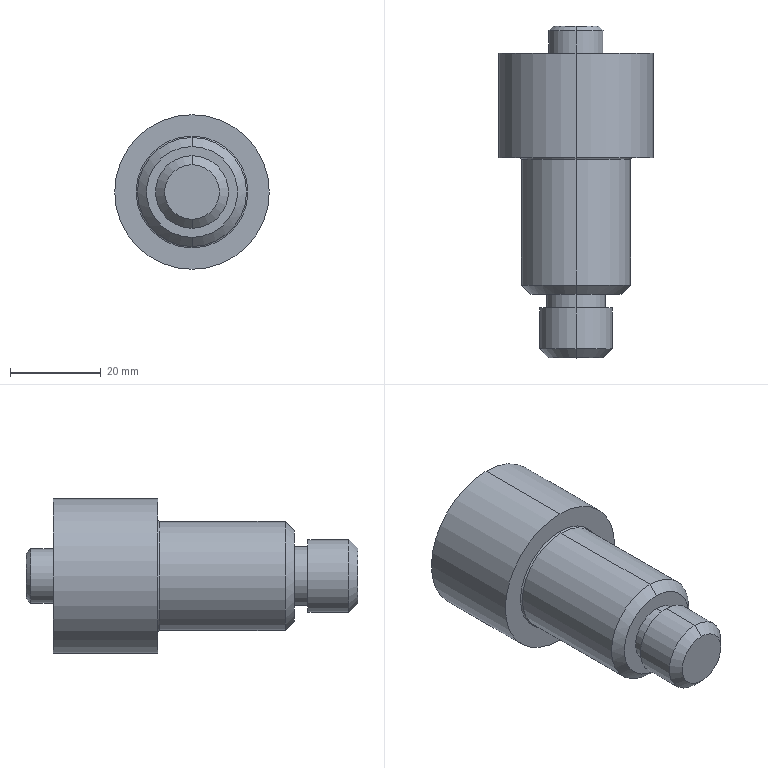Part | SolidWorks | features MirrorStock 1 | 1 solid | 24 faces | box 34 x 73 x 34 mm | volume 37491 mm3 | cylinder 10 | cone 6 | plane 6 | torus 2 | commonest cylinder face diameters 12 x2 13 x2 16 x2 24 x2 34 x2
STEP:
#1=CARTESIAN_POINT('',(0.,-29.3,12.));
#2=VERTEX_POINT('',#1);
#3=CARTESIAN_POINT('',(0.,-29.3,-12.));
#4=VERTEX_POINT('',#3);
#5=CARTESIAN_POINT('',(0.,-29.3,0.));
#6=DIRECTION('',(0.,1.,0.));
#7=DIRECTION('',(0.,0.,1.));
#8=AXIS2_PLACEMENT_3D('',#5,#6,#7);
#9=CIRCLE('',#8,12.);
#10=EDGE_CURVE('',#2,#4,#9,.T.);
#11=ORIENTED_EDGE('',*,*,#10,.T.);
#12=CARTESIAN_POINT('',(0.,-29.,-12.3));
#13=VERTEX_POINT('',#12);
#14=CARTESIAN_POINT('',(0.,-29.3,-12.3));
#15=DIRECTION('',(-1.,0.,0.));
#16=DIRECTION('',(0.,0.,1.));
#17=AXIS2_PLACEMENT_3D('',#14,#15,#16);
#18=CIRCLE('',#17,0.3);
#19=EDGE_CURVE('',#4,#13,#18,.T.);
#20=ORIENTED_EDGE('',*,*,#19,.T.);
#21=CARTESIAN_POINT('',(0.,-29.,12.3));
#22=VERTEX_POINT('',#21);
#23=CARTESIAN_POINT('',(0.,-29.,0.));
#24=DIRECTION('',(0.,-1.,0.));
#25=DIRECTION('',(0.,0.,1.));
#26=AXIS2_PLACEMENT_3D('',#23,#24,#25);
#27=CIRCLE('',#26,12.3);
#28=EDGE_CURVE('',#13,#22,#27,.T.);
#29=ORIENTED_EDGE('',*,*,#28,.T.);
#30=CARTESIAN_POINT('',(0.,-29.3,12.3));
#31=DIRECTION('',(1.,0.,0.));
#32=DIRECTION('',(0.,0.,-1.));
#33=AXIS2_PLACEMENT_3D('',#30,#31,#32);
#34=CIRCLE('',#33,0.3);
#35=EDGE_CURVE('',#2,#22,#34,.T.);
#36=ORIENTED_EDGE('',*,*,#35,.F.);
#37=EDGE_LOOP('',(#11,#20,#29,#36));
#38=FACE_OUTER_BOUND('',#37,.T.);
#39=CARTESIAN_POINT('',(0.,-29.3,0.));
#40=DIRECTION('',(0.,-1.,0.));
#41=DIRECTION('',(0.,0.,1.));
#42=AXIS2_PLACEMENT_3D('',#39,#40,#41);
#43=TOROIDAL_SURFACE('',#42,12.3,0.3);
#44=ADVANCED_FACE('',(#38),#43,.F.);
#45=CARTESIAN_POINT('',(0.,0.,5.));
#46=VERTEX_POINT('',#45);
#47=CARTESIAN_POINT('',(0.,0.,-5.));
#48=VERTEX_POINT('',#47);
#49=CARTESIAN_POINT('',(0.,0.,0.));
#50=DIRECTION('',(0.,-1.,0.));
#51=DIRECTION('',(0.,0.,-1.));
#52=AXIS2_PLACEMENT_3D('',#49,#50,#51);
#53=CIRCLE('',#52,5.);
#54=EDGE_CURVE('',#46,#48,#53,.T.);
#55=ORIENTED_EDGE('',*,*,#54,.T.);
#56=CARTESIAN_POINT('',(0.,-1.,-6.));
#57=VERTEX_POINT('',#56);
#58=CARTESIAN_POINT('',(0.,-1.,-6.));
#59=DIRECTION('',(0.,-0.7071,-0.7071));
#60=VECTOR('',#59,1000.);
#61=LINE('',#58,#60);
#62=EDGE_CURVE('',#48,#57,#61,.T.);
#63=ORIENTED_EDGE('',*,*,#62,.T.);
#64=CARTESIAN_POINT('',(0.,-1.,6.));
#65=VERTEX_POINT('',#64);
#66=CARTESIAN_POINT('',(0.,-1.,0.));
#67=DIRECTION('',(0.,1.,0.));
#68=DIRECTION('',(0.,0.,-1.));
#69=AXIS2_PLACEMENT_3D('',#66,#67,#68);
#70=CIRCLE('',#69,6.);
#71=EDGE_CURVE('',#57,#65,#70,.T.);
#72=ORIENTED_EDGE('',*,*,#71,.T.);
#73=CARTESIAN_POINT('',(0.,-1.,6.));
#74=DIRECTION('',(0.,-0.7071,0.7071));
#75=VECTOR('',#74,1000.);
#76=LINE('',#73,#75);
#77=EDGE_CURVE('',#46,#65,#76,.T.);
#78=ORIENTED_EDGE('',*,*,#77,.F.);
#79=EDGE_LOOP('',(#55,#63,#72,#78));
#80=FACE_OUTER_BOUND('',#79,.T.);
#81=CARTESIAN_POINT('',(0.,-1.,0.));
#82=DIRECTION('',(0.,-1.,0.));
#83=DIRECTION('',(0.,0.,1.));
#84=AXIS2_PLACEMENT_3D('',#81,#82,#83);
#85=CONICAL_SURFACE('',#84,6.,0.7854);
#86=ADVANCED_FACE('',(#80),#85,.T.);
#87=CARTESIAN_POINT('',(0.,-73.,-6.));
#88=VERTEX_POINT('',#87);
#89=CARTESIAN_POINT('',(0.,-73.,6.));
#90=VERTEX_POINT('',#89);
#91=CARTESIAN_POINT('',(0.,-73.,0.));
#92=DIRECTION('',(0.,1.,0.));
#93=DIRECTION('',(0.,0.,1.));
#94=AXIS2_PLACEMENT_3D('',#91,#92,#93);
#95=CIRCLE('',#94,6.);
#96=EDGE_CURVE('',#88,#90,#95,.T.);
#97=ORIENTED_EDGE('',*,*,#96,.T.);
#98=CARTESIAN_POINT('',(0.,-71.,8.));
#99=VERTEX_POINT('',#98);
#100=CARTESIAN_POINT('',(0.,-73.,6.));
#101=DIRECTION('',(0.,0.7071,0.7071));
#102=VECTOR('',#101,1000.);
#103=LINE('',#100,#102);
#104=EDGE_CURVE('',#90,#99,#103,.T.);
#105=ORIENTED_EDGE('',*,*,#104,.T.);
#106=CARTESIAN_POINT('',(0.,-71.,-8.));
#107=VERTEX_POINT('',#106);
#108=CARTESIAN_POINT('',(0.,-71.,0.));
#109=DIRECTION('',(0.,-1.,0.));
#110=DIRECTION('',(0.,0.,1.));
#111=AXIS2_PLACEMENT_3D('',#108,#109,#110);
#112=CIRCLE('',#111,8.);
#113=EDGE_CURVE('',#99,#107,#112,.T.);
#114=ORIENTED_EDGE('',*,*,#113,.T.);
#115=CARTESIAN_POINT('',(0.,-73.,-6.));
#116=DIRECTION('',(0.,0.7071,-0.7071));
#117=VECTOR('',#116,1000.);
#118=LINE('',#115,#117);
#119=EDGE_CURVE('',#88,#107,#118,.T.);
#120=ORIENTED_EDGE('',*,*,#119,.F.);
#121=EDGE_LOOP('',(#97,#105,#114,#120));
#122=FACE_OUTER_BOUND('',#121,.T.);
#123=CARTESIAN_POINT('',(0.,-73.,0.));
#124=DIRECTION('',(0.,1.,0.));
#125=DIRECTION('',(0.,0.,-1.));
#126=AXIS2_PLACEMENT_3D('',#123,#124,#125);
#127=CONICAL_SURFACE('',#126,6.,0.7854);
#128=ADVANCED_FACE('',(#122),#127,.T.);
#129=CARTESIAN_POINT('',(0.,-59.,-10.));
#130=VERTEX_POINT('',#129);
#131=CARTESIAN_POINT('',(0.,-59.,10.));
#132=VERTEX_POINT('',#131);
#133=CARTESIAN_POINT('',(0.,-59.,0.));
#134=DIRECTION('',(0.,1.,0.));
#135=DIRECTION('',(0.,0.,1.));
#136=AXIS2_PLACEMENT_3D('',#133,#134,#135);
#137=CIRCLE('',#136,10.);
#138=EDGE_CURVE('',#130,#132,#137,.T.);
#139=ORIENTED_EDGE('',*,*,#138,.T.);
#140=CARTESIAN_POINT('',(0.,-57.,12.));
#141=VERTEX_POINT('',#140);
#142=CARTESIAN_POINT('',(0.,-59.,10.));
#143=DIRECTION('',(0.,0.7071,0.7071));
#144=VECTOR('',#143,1000.);
#145=LINE('',#142,#144);
#146=EDGE_CURVE('',#132,#141,#145,.T.);
#147=ORIENTED_EDGE('',*,*,#146,.T.);
#148=CARTESIAN_POINT('',(0.,-57.,-12.));
#149=VERTEX_POINT('',#148);
#150=CARTESIAN_POINT('',(0.,-57.,0.));
#151=DIRECTION('',(0.,-1.,0.));
#152=DIRECTION('',(0.,0.,1.));
#153=AXIS2_PLACEMENT_3D('',#150,#151,#152);
#154=CIRCLE('',#153,12.);
#155=EDGE_CURVE('',#141,#149,#154,.T.);
#156=ORIENTED_EDGE('',*,*,#155,.T.);
#157=CARTESIAN_POINT('',(0.,-59.,-10.));
#158=DIRECTION('',(0.,0.7071,-0.7071));
#159=VECTOR('',#158,1000.);
#160=LINE('',#157,#159);
#161=EDGE_CURVE('',#130,#149,#160,.T.);
#162=ORIENTED_EDGE('',*,*,#161,.F.);
#163=EDGE_LOOP('',(#139,#147,#156,#162));
#164=FACE_OUTER_BOUND('',#163,.T.);
#165=CARTESIAN_POINT('',(0.,-59.,0.));
#166=DIRECTION('',(0.,1.,0.));
#167=DIRECTION('',(0.,0.,-1.));
#168=AXIS2_PLACEMENT_3D('',#165,#166,#167);
#169=CONICAL_SURFACE('',#168,10.,0.7854);
#170=ADVANCED_FACE('',(#164),#169,.T.);
#171=CARTESIAN_POINT('',(0.,-62.,-8.));
#172=VERTEX_POINT('',#171);
#173=CARTESIAN_POINT('',(0.,-62.,8.));
#174=VERTEX_POINT('',#173);
#175=CARTESIAN_POINT('',(0.,-62.,0.));
#176=DIRECTION('',(0.,1.,0.));
#177=DIRECTION('',(0.,0.,1.));
#178=AXIS2_PLACEMENT_3D('',#175,#176,#177);
#179=CIRCLE('',#178,8.);
#180=EDGE_CURVE('',#172,#174,#179,.T.);
#181=ORIENTED_EDGE('',*,*,#180,.F.);
#182=CARTESIAN_POINT('',(0.,-73.,-8.));
#183=DIRECTION('',(0.,-1.,0.));
#184=VECTOR('',#183,1000.);
#185=LINE('',#182,#184);
#186=EDGE_CURVE('',#172,#107,#185,.T.);
#187=ORIENTED_EDGE('',*,*,#186,.T.);
#188=ORIENTED_EDGE('',*,*,#113,.F.);
#189=CARTESIAN_POINT('',(0.,-73.,8.));
#190=DIRECTION('',(0.,-1.,0.));
#191=VECTOR('',#190,1000.);
#192=LINE('',#189,#191);
#193=EDGE_CURVE('',#174,#99,#192,.T.);
#194=ORIENTED_EDGE('',*,*,#193,.F.);
#195=EDGE_LOOP('',(#181,#187,#188,#194));
#196=FACE_OUTER_BOUND('',#195,.T.);
#197=CARTESIAN_POINT('',(0.,-73.,0.));
#198=DIRECTION('',(0.,-1.,0.));
#199=DIRECTION('',(0.,0.,1.));
#200=AXIS2_PLACEMENT_3D('',#197,#198,#199);
#201=CYLINDRICAL_SURFACE('',#200,8.);
#202=ADVANCED_FACE('',(#196),#201,.T.);
#203=CARTESIAN_POINT('',(0.,-59.,-6.5));
#204=VERTEX_POINT('',#203);
#205=CARTESIAN_POINT('',(0.,-59.,6.5));
#206=VERTEX_POINT('',#205);
#207=CARTESIAN_POINT('',(0.,-59.,0.));
#208=DIRECTION('',(0.,1.,0.));
#209=DIRECTION('',(0.,0.,1.));
#210=AXIS2_PLACEMENT_3D('',#207,#208,#209);
#211=CIRCLE('',#210,6.5);
#212=EDGE_CURVE('',#204,#206,#211,.T.);
#213=ORIENTED_EDGE('',*,*,#212,.F.);
#214=CARTESIAN_POINT('',(0.,-62.,-6.5));
#215=VERTEX_POINT('',#214);
#216=CARTESIAN_POINT('',(0.,-73.,-6.5));
#217=DIRECTION('',(0.,-1.,0.));
#218=VECTOR('',#217,1000.);
#219=LINE('',#216,#218);
#220=EDGE_CURVE('',#204,#215,#219,.T.);
#221=ORIENTED_EDGE('',*,*,#220,.T.);
#222=CARTESIAN_POINT('',(0.,-62.,6.5));
#223=VERTEX_POINT('',#222);
#224=CARTESIAN_POINT('',(0.,-62.,0.));
#225=DIRECTION('',(0.,1.,0.));
#226=DIRECTION('',(0.,0.,1.));
#227=AXIS2_PLACEMENT_3D('',#224,#225,#226);
#228=CIRCLE('',#227,6.5);
#229=EDGE_CURVE('',#215,#223,#228,.T.);
#230=ORIENTED_EDGE('',*,*,#229,.T.);
#231=CARTESIAN_POINT('',(0.,-73.,6.5));
#232=DIRECTION('',(0.,-1.,0.));
#233=VECTOR('',#232,1000.);
#234=LINE('',#231,#233);
#235=EDGE_CURVE('',#206,#223,#234,.T.);
#236=ORIENTED_EDGE('',*,*,#235,.F.);
#237=EDGE_LOOP('',(#213,#221,#230,#236));
#238=FACE_OUTER_BOUND('',#237,.T.);
#239=CARTESIAN_POINT('',(0.,-73.,0.));
#240=DIRECTION('',(0.,-1.,0.));
#241=DIRECTION('',(0.,0.,1.));
#242=AXIS2_PLACEMENT_3D('',#239,#240,#241);
#243=CYLINDRICAL_SURFACE('',#242,6.5);
#244=ADVANCED_FACE('',(#238),#243,.T.);
#245=CARTESIAN_POINT('',(0.,-29.3,0.));
#246=DIRECTION('',(0.,1.,0.));
#247=DIRECTION('',(0.,0.,1.));
#248=AXIS2_PLACEMENT_3D('',#245,#246,#247);
#249=CIRCLE('',#248,12.);
#250=EDGE_CURVE('',#4,#2,#249,.T.);
#251=ORIENTED_EDGE('',*,*,#250,.F.);
#252=CARTESIAN_POINT('',(0.,-73.,-12.));
#253=DIRECTION('',(0.,-1.,0.));
#254=VECTOR('',#253,1000.);
#255=LINE('',#252,#254);
#256=EDGE_CURVE('',#4,#149,#255,.T.);
#257=ORIENTED_EDGE('',*,*,#256,.T.);
#258=ORIENTED_EDGE('',*,*,#155,.F.);
#259=CARTESIAN_POINT('',(0.,-73.,12.));
#260=DIRECTION('',(0.,-1.,0.));
#261=VECTOR('',#260,1000.);
#262=LINE('',#259,#261);
#263=EDGE_CURVE('',#2,#141,#262,.T.);
#264=ORIENTED_EDGE('',*,*,#263,.F.);
#265=EDGE_LOOP('',(#251,#257,#258,#264));
#266=FACE_OUTER_BOUND('',#265,.T.);
#267=CARTESIAN_POINT('',(0.,-73.,0.));
#268=DIRECTION('',(0.,-1.,0.));
#269=DIRECTION('',(0.,0.,1.));
#270=AXIS2_PLACEMENT_3D('',#267,#268,#269);
#271=CYLINDRICAL_SURFACE('',#270,12.);
#272=ADVANCED_FACE('',(#266),#271,.T.);
#273=CARTESIAN_POINT('',(0.,-6.,-17.));
#274=VERTEX_POINT('',#273);
#275=CARTESIAN_POINT('',(0.,-6.,17.));
#276=VERTEX_POINT('',#275);
#277=CARTESIAN_POINT('',(0.,-6.,0.));
#278=DIRECTION('',(0.,1.,0.));
#279=DIRECTION('',(0.,0.,1.));
#280=AXIS2_PLACEMENT_3D('',#277,#278,#279);
#281=CIRCLE('',#280,17.);
#282=EDGE_CURVE('',#274,#276,#281,.T.);
#283=ORIENTED_EDGE('',*,*,#282,.F.);
#284=CARTESIAN_POINT('',(0.,-29.,-17.));
#285=VERTEX_POINT('',#284);
#286=CARTESIAN_POINT('',(0.,-73.,-17.));
#287=DIRECTION('',(0.,-1.,0.));
#288=VECTOR('',#287,1000.);
#289=LINE('',#286,#288);
#290=EDGE_CURVE('',#274,#285,#289,.T.);
#291=ORIENTED_EDGE('',*,*,#290,.T.);
#292=CARTESIAN_POINT('',(0.,-29.,17.));
#293=VERTEX_POINT('',#292);
#294=CARTESIAN_POINT('',(0.,-29.,0.));
#295=DIRECTION('',(0.,1.,0.));
#296=DIRECTION('',(0.,0.,1.));
#297=AXIS2_PLACEMENT_3D('',#294,#295,#296);
#298=CIRCLE('',#297,17.);
#299=EDGE_CURVE('',#285,#293,#298,.T.);
#300=ORIENTED_EDGE('',*,*,#299,.T.);
#301=CARTESIAN_POINT('',(0.,-73.,17.));
#302=DIRECTION('',(0.,-1.,0.));
#303=VECTOR('',#302,1000.);
#304=LINE('',#301,#303);
#305=EDGE_CURVE('',#276,#293,#304,.T.);
#306=ORIENTED_EDGE('',*,*,#305,.F.);
#307=EDGE_LOOP('',(#283,#291,#300,#306));
#308=FACE_OUTER_BOUND('',#307,.T.);
#309=CARTESIAN_POINT('',(0.,-73.,0.));
#310=DIRECTION('',(0.,-1.,0.));
#311=DIRECTION('',(0.,0.,1.));
#312=AXIS2_PLACEMENT_3D('',#309,#310,#311);
#313=CYLINDRICAL_SURFACE('',#312,17.);
#314=ADVANCED_FACE('',(#308),#313,.T.);
#315=ORIENTED_EDGE('',*,*,#71,.F.);
#316=CARTESIAN_POINT('',(0.,-6.,-6.));
#317=VERTEX_POINT('',#316);
#318=CARTESIAN_POINT('',(0.,-73.,-6.));
#319=DIRECTION('',(0.,-1.,0.));
#320=VECTOR('',#319,1000.);
#321=LINE('',#318,#320);
#322=EDGE_CURVE('',#57,#317,#321,.T.);
#323=ORIENTED_EDGE('',*,*,#322,.T.);
#324=CARTESIAN_POINT('',(0.,-6.,6.));
#325=VERTEX_POINT('',#324);
#326=CARTESIAN_POINT('',(0.,-6.,0.));
#327=DIRECTION('',(0.,1.,0.));
#328=DIRECTION('',(0.,0.,1.));
#329=AXIS2_PLACEMENT_3D('',#326,#327,#328);
#330=CIRCLE('',#329,6.);
#331=EDGE_CURVE('',#317,#325,#330,.T.);
#332=ORIENTED_EDGE('',*,*,#331,.T.);
#333=CARTESIAN_POINT('',(0.,-73.,6.));
#334=DIRECTION('',(0.,-1.,0.));
#335=VECTOR('',#334,1000.);
#336=LINE('',#333,#335);
#337=EDGE_CURVE('',#65,#325,#336,.T.);
#338=ORIENTED_EDGE('',*,*,#337,.F.);
#339=EDGE_LOOP('',(#315,#323,#332,#338));
#340=FACE_OUTER_BOUND('',#339,.T.);
#341=CARTESIAN_POINT('',(0.,-73.,0.));
#342=DIRECTION('',(0.,-1.,0.));
#343=DIRECTION('',(0.,0.,1.));
#344=AXIS2_PLACEMENT_3D('',#341,#342,#343);
#345=CYLINDRICAL_SURFACE('',#344,6.);
#346=ADVANCED_FACE('',(#340),#345,.T.);
#347=ORIENTED_EDGE('',*,*,#54,.F.);
#348=CARTESIAN_POINT('',(0.,0.,0.));
#349=DIRECTION('',(0.,-1.,0.));
#350=DIRECTION('',(0.,0.,-1.));
#351=AXIS2_PLACEMENT_3D('',#348,#349,#350);
#352=CIRCLE('',#351,5.);
#353=EDGE_CURVE('',#48,#46,#352,.T.);
#354=ORIENTED_EDGE('',*,*,#353,.F.);
#355=EDGE_LOOP('',(#347,#354));
#356=FACE_OUTER_BOUND('',#355,.T.);
#357=CARTESIAN_POINT('',(0.,0.,0.));
#358=DIRECTION('',(0.,1.,0.));
#359=DIRECTION('',(0.,0.,-1.));
#360=AXIS2_PLACEMENT_3D('',#357,#358,#359);
#361=PLANE('',#360);
#362=ADVANCED_FACE('',(#356),#361,.T.);
#363=ORIENTED_EDGE('',*,*,#322,.F.);
#364=CARTESIAN_POINT('',(0.,-1.,0.));
#365=DIRECTION('',(0.,1.,0.));
#366=DIRECTION('',(0.,0.,-1.));
#367=AXIS2_PLACEMENT_3D('',#364,#365,#366);
#368=CIRCLE('',#367,6.);
#369=EDGE_CURVE('',#65,#57,#368,.T.);
#370=ORIENTED_EDGE('',*,*,#369,.F.);
#371=ORIENTED_EDGE('',*,*,#337,.T.);
#372=CARTESIAN_POINT('',(0.,-6.,0.));
#373=DIRECTION('',(0.,1.,0.));
#374=DIRECTION('',(0.,0.,1.));
#375=AXIS2_PLACEMENT_3D('',#372,#373,#374);
#376=CIRCLE('',#375,6.);
#377=EDGE_CURVE('',#325,#317,#376,.T.);
#378=ORIENTED_EDGE('',*,*,#377,.T.);
#379=EDGE_LOOP('',(#363,#370,#371,#378));
#380=FACE_OUTER_BOUND('',#379,.T.);
#381=CARTESIAN_POINT('',(0.,-73.,0.));
#382=DIRECTION('',(0.,-1.,0.));
#383=DIRECTION('',(0.,0.,1.));
#384=AXIS2_PLACEMENT_3D('',#381,#382,#383);
#385=CYLINDRICAL_SURFACE('',#384,6.);
#386=ADVANCED_FACE('',(#380),#385,.T.);
#387=ORIENTED_EDGE('',*,*,#377,.F.);
#388=ORIENTED_EDGE('',*,*,#331,.F.);
#389=EDGE_LOOP('',(#387,#388));
#390=FACE_BOUND('',#389,.T.);
#391=CARTESIAN_POINT('',(0.,-6.,0.));
#392=DIRECTION('',(0.,1.,0.));
#393=DIRECTION('',(0.,0.,1.));
#394=AXIS2_PLACEMENT_3D('',#391,#392,#393);
#395=CIRCLE('',#394,17.);
#396=EDGE_CURVE('',#276,#274,#395,.T.);
#397=ORIENTED_EDGE('',*,*,#396,.T.);
#398=ORIENTED_EDGE('',*,*,#282,.T.);
#399=EDGE_LOOP('',(#397,#398));
#400=FACE_OUTER_BOUND('',#399,.T.);
#401=CARTESIAN_POINT('',(6.,-6.,0.));
#402=DIRECTION('',(0.,1.,0.));
#403=DIRECTION('',(0.,0.,-1.));
#404=AXIS2_PLACEMENT_3D('',#401,#402,#403);
#405=PLANE('',#404);
#406=ADVANCED_FACE('',(#390,#400),#405,.T.);
#407=ORIENTED_EDGE('',*,*,#290,.F.);
#408=ORIENTED_EDGE('',*,*,#396,.F.);
#409=ORIENTED_EDGE('',*,*,#305,.T.);
#410=CARTESIAN_POINT('',(0.,-29.,0.));
#411=DIRECTION('',(0.,1.,0.));
#412=DIRECTION('',(0.,0.,1.));
#413=AXIS2_PLACEMENT_3D('',#410,#411,#412);
#414=CIRCLE('',#413,17.);
#415=EDGE_CURVE('',#293,#285,#414,.T.);
#416=ORIENTED_EDGE('',*,*,#415,.T.);
#417=EDGE_LOOP('',(#407,#408,#409,#416));
#418=FACE_OUTER_BOUND('',#417,.T.);
#419=CARTESIAN_POINT('',(0.,-73.,0.));
#420=DIRECTION('',(0.,-1.,0.));
#421=DIRECTION('',(0.,0.,1.));
#422=AXIS2_PLACEMENT_3D('',#419,#420,#421);
#423=CYLINDRICAL_SURFACE('',#422,17.);
#424=ADVANCED_FACE('',(#418),#423,.T.);
#425=CARTESIAN_POINT('',(0.,-29.,0.));
#426=DIRECTION('',(0.,-1.,0.));
#427=DIRECTION('',(0.,0.,1.));
#428=AXIS2_PLACEMENT_3D('',#425,#426,#427);
#429=CIRCLE('',#428,12.3);
#430=EDGE_CURVE('',#22,#13,#429,.T.);
#431=ORIENTED_EDGE('',*,*,#430,.F.);
#432=ORIENTED_EDGE('',*,*,#28,.F.);
#433=EDGE_LOOP('',(#431,#432));
#434=FACE_BOUND('',#433,.T.);
#435=ORIENTED_EDGE('',*,*,#415,.F.);
#436=ORIENTED_EDGE('',*,*,#299,.F.);
#437=EDGE_LOOP('',(#435,#436));
#438=FACE_OUTER_BOUND('',#437,.T.);
#439=CARTESIAN_POINT('',(17.,-29.,0.));
#440=DIRECTION('',(0.,-1.,0.));
#441=DIRECTION('',(0.,0.,1.));
#442=AXIS2_PLACEMENT_3D('',#439,#440,#441);
#443=PLANE('',#442);
#444=ADVANCED_FACE('',(#434,#438),#443,.T.);
#445=ORIENTED_EDGE('',*,*,#256,.F.);
#446=ORIENTED_EDGE('',*,*,#10,.F.);
#447=ORIENTED_EDGE('',*,*,#263,.T.);
#448=CARTESIAN_POINT('',(0.,-57.,0.));
#449=DIRECTION('',(0.,-1.,0.));
#450=DIRECTION('',(0.,0.,1.));
#451=AXIS2_PLACEMENT_3D('',#448,#449,#450);
#452=CIRCLE('',#451,12.);
#453=EDGE_CURVE('',#149,#141,#452,.T.);
#454=ORIENTED_EDGE('',*,*,#453,.F.);
#455=EDGE_LOOP('',(#445,#446,#447,#454));
#456=FACE_OUTER_BOUND('',#455,.T.);
#457=CARTESIAN_POINT('',(0.,-73.,0.));
#458=DIRECTION('',(0.,-1.,0.));
#459=DIRECTION('',(0.,0.,1.));
#460=AXIS2_PLACEMENT_3D('',#457,#458,#459);
#461=CYLINDRICAL_SURFACE('',#460,12.);
#462=ADVANCED_FACE('',(#456),#461,.T.);
#463=ORIENTED_EDGE('',*,*,#138,.F.);
#464=CARTESIAN_POINT('',(0.,-59.,0.));
#465=DIRECTION('',(0.,1.,0.));
#466=DIRECTION('',(0.,0.,1.));
#467=AXIS2_PLACEMENT_3D('',#464,#465,#466);
#468=CIRCLE('',#467,10.);
#469=EDGE_CURVE('',#132,#130,#468,.T.);
#470=ORIENTED_EDGE('',*,*,#469,.F.);
#471=EDGE_LOOP('',(#463,#470));
#472=FACE_OUTER_BOUND('',#471,.T.);
#473=CARTESIAN_POINT('',(0.,-59.,0.));
#474=DIRECTION('',(0.,1.,0.));
#475=DIRECTION('',(0.,0.,1.));
#476=AXIS2_PLACEMENT_3D('',#473,#474,#475);
#477=CIRCLE('',#476,6.5);
#478=EDGE_CURVE('',#206,#204,#477,.T.);
#479=ORIENTED_EDGE('',*,*,#478,.T.);
#480=ORIENTED_EDGE('',*,*,#212,.T.);
#481=EDGE_LOOP('',(#479,#480));
#482=FACE_BOUND('',#481,.T.);
#483=CARTESIAN_POINT('',(12.,-59.,0.));
#484=DIRECTION('',(0.,-1.,0.));
#485=DIRECTION('',(0.,0.,1.));
#486=AXIS2_PLACEMENT_3D('',#483,#484,#485);
#487=PLANE('',#486);
#488=ADVANCED_FACE('',(#472,#482),#487,.T.);
#489=ORIENTED_EDGE('',*,*,#220,.F.);
#490=ORIENTED_EDGE('',*,*,#478,.F.);
#491=ORIENTED_EDGE('',*,*,#235,.T.);
#492=CARTESIAN_POINT('',(0.,-62.,0.));
#493=DIRECTION('',(0.,1.,0.));
#494=DIRECTION('',(0.,0.,1.));
#495=AXIS2_PLACEMENT_3D('',#492,#493,#494);
#496=CIRCLE('',#495,6.5);
#497=EDGE_CURVE('',#223,#215,#496,.T.);
#498=ORIENTED_EDGE('',*,*,#497,.T.);
#499=EDGE_LOOP('',(#489,#490,#491,#498));
#500=FACE_OUTER_BOUND('',#499,.T.);
#501=CARTESIAN_POINT('',(0.,-73.,0.));
#502=DIRECTION('',(0.,-1.,0.));
#503=DIRECTION('',(0.,0.,1.));
#504=AXIS2_PLACEMENT_3D('',#501,#502,#503);
#505=CYLINDRICAL_SURFACE('',#504,6.5);
#506=ADVANCED_FACE('',(#500),#505,.T.);
#507=ORIENTED_EDGE('',*,*,#497,.F.);
#508=ORIENTED_EDGE('',*,*,#229,.F.);
#509=EDGE_LOOP('',(#507,#508));
#510=FACE_BOUND('',#509,.T.);
#511=CARTESIAN_POINT('',(0.,-62.,0.));
#512=DIRECTION('',(0.,1.,0.));
#513=DIRECTION('',(0.,0.,1.));
#514=AXIS2_PLACEMENT_3D('',#511,#512,#513);
#515=CIRCLE('',#514,8.);
#516=EDGE_CURVE('',#174,#172,#515,.T.);
#517=ORIENTED_EDGE('',*,*,#516,.T.);
#518=ORIENTED_EDGE('',*,*,#180,.T.);
#519=EDGE_LOOP('',(#517,#518));
#520=FACE_OUTER_BOUND('',#519,.T.);
#521=CARTESIAN_POINT('',(6.5,-62.,0.));
#522=DIRECTION('',(0.,1.,0.));
#523=DIRECTION('',(0.,0.,-1.));
#524=AXIS2_PLACEMENT_3D('',#521,#522,#523);
#525=PLANE('',#524);
#526=ADVANCED_FACE('',(#510,#520),#525,.T.);
#527=ORIENTED_EDGE('',*,*,#186,.F.);
#528=ORIENTED_EDGE('',*,*,#516,.F.);
#529=ORIENTED_EDGE('',*,*,#193,.T.);
#530=CARTESIAN_POINT('',(0.,-71.,0.));
#531=DIRECTION('',(0.,-1.,0.));
#532=DIRECTION('',(0.,0.,1.));
#533=AXIS2_PLACEMENT_3D('',#530,#531,#532);
#534=CIRCLE('',#533,8.);
#535=EDGE_CURVE('',#107,#99,#534,.T.);
#536=ORIENTED_EDGE('',*,*,#535,.F.);
#537=EDGE_LOOP('',(#527,#528,#529,#536));
#538=FACE_OUTER_BOUND('',#537,.T.);
#539=CARTESIAN_POINT('',(0.,-73.,0.));
#540=DIRECTION('',(0.,-1.,0.));
#541=DIRECTION('',(0.,0.,1.));
#542=AXIS2_PLACEMENT_3D('',#539,#540,#541);
#543=CYLINDRICAL_SURFACE('',#542,8.);
#544=ADVANCED_FACE('',(#538),#543,.T.);
#545=ORIENTED_EDGE('',*,*,#96,.F.);
#546=CARTESIAN_POINT('',(0.,-73.,0.));
#547=DIRECTION('',(0.,1.,0.));
#548=DIRECTION('',(0.,0.,1.));
#549=AXIS2_PLACEMENT_3D('',#546,#547,#548);
#550=CIRCLE('',#549,6.);
#551=EDGE_CURVE('',#90,#88,#550,.T.);
#552=ORIENTED_EDGE('',*,*,#551,.F.);
#553=EDGE_LOOP('',(#545,#552));
#554=FACE_OUTER_BOUND('',#553,.T.);
#555=CARTESIAN_POINT('',(8.,-73.,0.));
#556=DIRECTION('',(0.,-1.,0.));
#557=DIRECTION('',(0.,0.,1.));
#558=AXIS2_PLACEMENT_3D('',#555,#556,#557);
#559=PLANE('',#558);
#560=ADVANCED_FACE('',(#554),#559,.T.);
#561=ORIENTED_EDGE('',*,*,#146,.F.);
#562=ORIENTED_EDGE('',*,*,#469,.T.);
#563=ORIENTED_EDGE('',*,*,#161,.T.);
#564=ORIENTED_EDGE('',*,*,#453,.T.);
#565=EDGE_LOOP('',(#561,#562,#563,#564));
#566=FACE_OUTER_BOUND('',#565,.T.);
#567=CARTESIAN_POINT('',(0.,-59.,0.));
#568=DIRECTION('',(0.,1.,0.));
#569=DIRECTION('',(0.,0.,-1.));
#570=AXIS2_PLACEMENT_3D('',#567,#568,#569);
#571=CONICAL_SURFACE('',#570,10.,0.7854);
#572=ADVANCED_FACE('',(#566),#571,.T.);
#573=ORIENTED_EDGE('',*,*,#104,.F.);
#574=ORIENTED_EDGE('',*,*,#551,.T.);
#575=ORIENTED_EDGE('',*,*,#119,.T.);
#576=ORIENTED_EDGE('',*,*,#535,.T.);
#577=EDGE_LOOP('',(#573,#574,#575,#576));
#578=FACE_OUTER_BOUND('',#577,.T.);
#579=CARTESIAN_POINT('',(0.,-73.,0.));
#580=DIRECTION('',(0.,1.,0.));
#581=DIRECTION('',(0.,0.,-1.));
#582=AXIS2_PLACEMENT_3D('',#579,#580,#581);
#583=CONICAL_SURFACE('',#582,6.,0.7854);
#584=ADVANCED_FACE('',(#578),#583,.T.);
#585=ORIENTED_EDGE('',*,*,#62,.F.);
#586=ORIENTED_EDGE('',*,*,#353,.T.);
#587=ORIENTED_EDGE('',*,*,#77,.T.);
#588=ORIENTED_EDGE('',*,*,#369,.T.);
#589=EDGE_LOOP('',(#585,#586,#587,#588));
#590=FACE_OUTER_BOUND('',#589,.T.);
#591=CARTESIAN_POINT('',(0.,-1.,0.));
#592=DIRECTION('',(0.,-1.,0.));
#593=DIRECTION('',(0.,0.,1.));
#594=AXIS2_PLACEMENT_3D('',#591,#592,#593);
#595=CONICAL_SURFACE('',#594,6.,0.7854);
#596=ADVANCED_FACE('',(#590),#595,.T.);
#597=ORIENTED_EDGE('',*,*,#19,.F.);
#598=ORIENTED_EDGE('',*,*,#250,.T.);
#599=ORIENTED_EDGE('',*,*,#35,.T.);
#600=ORIENTED_EDGE('',*,*,#430,.T.);
#601=EDGE_LOOP('',(#597,#598,#599,#600));
#602=FACE_OUTER_BOUND('',#601,.T.);
#603=CARTESIAN_POINT('',(0.,-29.3,0.));
#604=DIRECTION('',(0.,-1.,0.));
#605=DIRECTION('',(0.,0.,1.));
#606=AXIS2_PLACEMENT_3D('',#603,#604,#605);
#607=TOROIDAL_SURFACE('',#606,12.3,0.3);
#608=ADVANCED_FACE('',(#602),#607,.F.);
#609=CLOSED_SHELL('',(#44,#86,#128,#170,#202,#244,#272,#314,#346,#362,#386,#406,#424,#444,#462,#488,#506,#526,#544,#560,#572,#584,#596,#608));
#610=MANIFOLD_SOLID_BREP('',#609);
#611=CARTESIAN_POINT('',(0.,0.,0.));
#612=DIRECTION('',(0.,0.,1.));
#613=DIRECTION('',(1.,0.,0.));
#614=AXIS2_PLACEMENT_3D('',#611,#612,#613);
#615=(LENGTH_UNIT()NAMED_UNIT(*)SI_UNIT(.MILLI.,.METRE.));
#616=UNCERTAINTY_MEASURE_WITH_UNIT(LENGTH_MEASURE(0.00001),#615,'','');
#617=(NAMED_UNIT(*)PLANE_ANGLE_UNIT()SI_UNIT($,.RADIAN.));
#618=(NAMED_UNIT(*)SI_UNIT($,.STERADIAN.)SOLID_ANGLE_UNIT());
#619=(GEOMETRIC_REPRESENTATION_CONTEXT(3)GLOBAL_UNCERTAINTY_ASSIGNED_CONTEXT((#616))GLOBAL_UNIT_ASSIGNED_CONTEXT((#615,#617,#618))REPRESENTATION_CONTEXT('',''));
#620=ADVANCED_BREP_SHAPE_REPRESENTATION('',(#610,#614),#619);